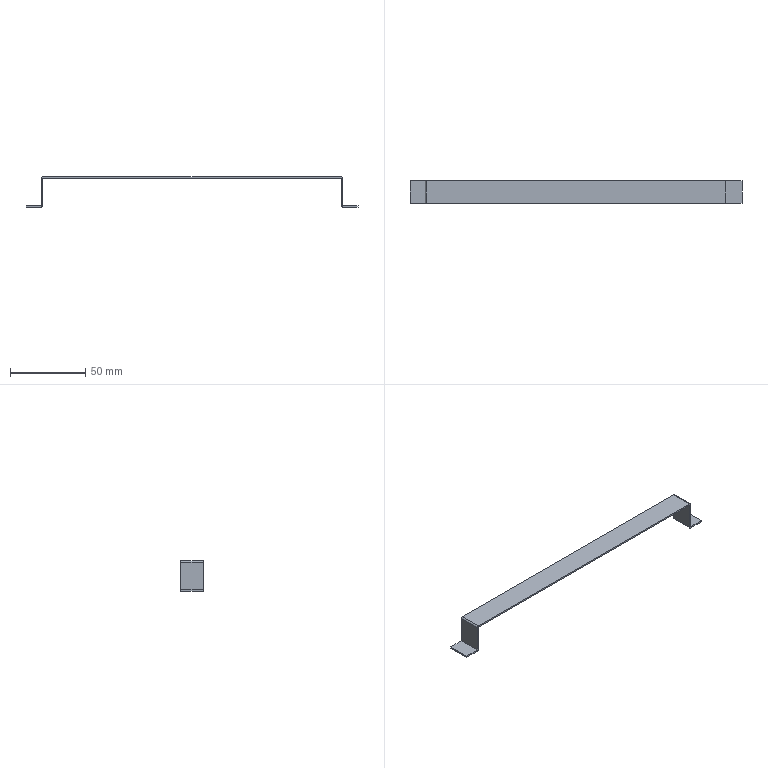Part | STEP file | RJWD-DY-0101_0003 | 1 solid | 18 faces | box 220 x 15 x 20 mm | volume 3858 mm3 | plane 14 | cylinder 4 | commonest cylinder face diameters 2.004 x4
STEP:
#1=CARTESIAN_POINT('',(0.,0.,0.));
#2=DIRECTION('',(0.,0.,1.));
#3=DIRECTION('',(1.,0.,0.));
#4=AXIS2_PLACEMENT_3D('',#1,#2,#3);
#5=CARTESIAN_POINT('',(-779.572,5371.573,97.643));
#6=VERTEX_POINT('',#5);
#7=CARTESIAN_POINT('',(-779.573,5371.573,79.646));
#8=VERTEX_POINT('',#7);
#9=CARTESIAN_POINT('',(-779.572,5371.573,97.643));
#10=DIRECTION('',(-0.00003704,0.,-1.));
#11=VECTOR('',#10,1.);
#12=LINE('',#9,#11);
#13=CARTESIAN_POINT('',(-560.573,5371.573,97.644));
#14=DIRECTION('',(0.,-1.,0.));
#15=DIRECTION('',(0.,0.,-1.));
#16=AXIS2_PLACEMENT_3D('',#13,#14,#15);
#17=PLANE('',#16);
#18=CARTESIAN_POINT('',(0.0006667,-218.999));
#19=DIRECTION('',(1.,-0.00003704));
#20=VECTOR('',#19,1.);
#21=LINE('',#18,#20);
#22=(GEOMETRIC_REPRESENTATION_CONTEXT(2)PARAMETRIC_REPRESENTATION_CONTEXT()REPRESENTATION_CONTEXT('',''));
#23=DEFINITIONAL_REPRESENTATION('',(#21),#22);
#24=PCURVE('',#17,#23);
#25=CARTESIAN_POINT('',(-779.573,-10.,0.));
#26=DIRECTION('',(-1.,0.,0.));
#27=DIRECTION('',(0.,0.,-1.));
#28=AXIS2_PLACEMENT_3D('',#25,#26,#27);
#29=PLANE('',#28);
#30=CARTESIAN_POINT('',(-97.643,-5381.573));
#31=DIRECTION('',(1.,0.));
#32=VECTOR('',#31,1.);
#33=LINE('',#30,#32);
#34=(GEOMETRIC_REPRESENTATION_CONTEXT(2)PARAMETRIC_REPRESENTATION_CONTEXT()REPRESENTATION_CONTEXT('',''));
#35=DEFINITIONAL_REPRESENTATION('',(#33),#34);
#36=PCURVE('',#29,#35);
#37=SURFACE_CURVE('',#12,(#24,#36),.PCURVE_S1.);
#38=EDGE_CURVE('',#6,#8,#37,.T.);
#39=ORIENTED_EDGE('',*,*,#38,.T.);
#40=CARTESIAN_POINT('',(-780.575,5371.573,78.644));
#41=VERTEX_POINT('',#40);
#42=CARTESIAN_POINT('',(-780.575,5371.573,79.646));
#43=DIRECTION('',(0.,-1.,0.));
#44=DIRECTION('',(0.,0.,-1.));
#45=AXIS2_PLACEMENT_3D('',#42,#43,#44);
#46=CIRCLE('',#45,1.002);
#47=CARTESIAN_POINT('',(17.998,-220.002));
#48=DIRECTION('',(1.,0.));
#49=AXIS2_PLACEMENT_2D('',#47,#48);
#50=CIRCLE('',#49,1.002);
#51=(GEOMETRIC_REPRESENTATION_CONTEXT(2)PARAMETRIC_REPRESENTATION_CONTEXT()REPRESENTATION_CONTEXT('',''));
#52=DEFINITIONAL_REPRESENTATION('',(#50),#51);
#53=PCURVE('',#17,#52);
#54=CARTESIAN_POINT('',(-780.575,5411.573,79.646));
#55=DIRECTION('',(0.,-1.,0.));
#56=DIRECTION('',(-1.,0.,0.));
#57=AXIS2_PLACEMENT_3D('',#54,#55,#56);
#58=CYLINDRICAL_SURFACE('',#57,1.002);
#59=CARTESIAN_POINT('',(1.571,40.));
#60=DIRECTION('',(1.,0.));
#61=VECTOR('',#60,1.);
#62=LINE('',#59,#61);
#63=(GEOMETRIC_REPRESENTATION_CONTEXT(2)PARAMETRIC_REPRESENTATION_CONTEXT()REPRESENTATION_CONTEXT('',''));
#64=DEFINITIONAL_REPRESENTATION('',(#62),#63);
#65=PCURVE('',#58,#64);
#66=SURFACE_CURVE('',#46,(#53,#65),.PCURVE_S1.);
#67=EDGE_CURVE('',#41,#8,#66,.T.);
#68=ORIENTED_EDGE('',*,*,#67,.F.);
#69=CARTESIAN_POINT('',(-790.573,5371.573,78.644));
#70=VERTEX_POINT('',#69);
#71=CARTESIAN_POINT('',(-780.575,5371.573,78.644));
#72=DIRECTION('',(-1.,0.,0.));
#73=VECTOR('',#72,1.);
#74=LINE('',#71,#73);
#75=CARTESIAN_POINT('',(19.,-220.002));
#76=DIRECTION('',(0.,-1.));
#77=VECTOR('',#76,1.);
#78=LINE('',#75,#77);
#79=(GEOMETRIC_REPRESENTATION_CONTEXT(2)PARAMETRIC_REPRESENTATION_CONTEXT()REPRESENTATION_CONTEXT('',''));
#80=DEFINITIONAL_REPRESENTATION('',(#78),#79);
#81=PCURVE('',#17,#80);
#82=CARTESIAN_POINT('',(-1601.145,-10.,78.644));
#83=DIRECTION('',(0.,0.,1.));
#84=DIRECTION('',(-1.,0.,0.));
#85=AXIS2_PLACEMENT_3D('',#82,#83,#84);
#86=PLANE('',#85);
#87=CARTESIAN_POINT('',(-820.571,-5381.573));
#88=DIRECTION('',(1.,0.));
#89=VECTOR('',#88,1.);
#90=LINE('',#87,#89);
#91=(GEOMETRIC_REPRESENTATION_CONTEXT(2)PARAMETRIC_REPRESENTATION_CONTEXT()REPRESENTATION_CONTEXT('',''));
#92=DEFINITIONAL_REPRESENTATION('',(#90),#91);
#93=PCURVE('',#86,#92);
#94=SURFACE_CURVE('',#74,(#81,#93),.PCURVE_S1.);
#95=EDGE_CURVE('',#41,#70,#94,.T.);
#96=ORIENTED_EDGE('',*,*,#95,.T.);
#97=CARTESIAN_POINT('',(-790.573,5371.573,79.644));
#98=VERTEX_POINT('',#97);
#99=CARTESIAN_POINT('',(-790.573,5371.573,78.644));
#100=DIRECTION('',(0.,0.,1.));
#101=VECTOR('',#100,1.);
#102=LINE('',#99,#101);
#103=CARTESIAN_POINT('',(19.,-230.));
#104=DIRECTION('',(-1.,0.));
#105=VECTOR('',#104,1.);
#106=LINE('',#103,#105);
#107=(GEOMETRIC_REPRESENTATION_CONTEXT(2)PARAMETRIC_REPRESENTATION_CONTEXT()REPRESENTATION_CONTEXT('',''));
#108=DEFINITIONAL_REPRESENTATION('',(#106),#107);
#109=PCURVE('',#17,#108);
#110=CARTESIAN_POINT('',(-790.573,5371.573,78.644));
#111=DIRECTION('',(-1.,0.,0.));
#112=DIRECTION('',(0.,0.,-1.));
#113=AXIS2_PLACEMENT_3D('',#110,#111,#112);
#114=PLANE('',#113);
#115=CARTESIAN_POINT('',(0.,0.));
#116=DIRECTION('',(-1.,0.));
#117=VECTOR('',#116,1.);
#118=LINE('',#115,#117);
#119=(GEOMETRIC_REPRESENTATION_CONTEXT(2)PARAMETRIC_REPRESENTATION_CONTEXT()REPRESENTATION_CONTEXT('',''));
#120=DEFINITIONAL_REPRESENTATION('',(#118),#119);
#121=PCURVE('',#114,#120);
#122=SURFACE_CURVE('',#102,(#109,#121),.PCURVE_S1.);
#123=EDGE_CURVE('',#70,#98,#122,.T.);
#124=ORIENTED_EDGE('',*,*,#123,.T.);
#125=CARTESIAN_POINT('',(-780.573,5371.573,79.644));
#126=VERTEX_POINT('',#125);
#127=CARTESIAN_POINT('',(-780.573,5371.573,79.644));
#128=DIRECTION('',(-1.,0.,-0.00006667));
#129=VECTOR('',#128,1.);
#130=LINE('',#127,#129);
#131=CARTESIAN_POINT('',(17.999,-220.001));
#132=DIRECTION('',(0.00006667,-1.));
#133=VECTOR('',#132,1.);
#134=LINE('',#131,#133);
#135=(GEOMETRIC_REPRESENTATION_CONTEXT(2)PARAMETRIC_REPRESENTATION_CONTEXT()REPRESENTATION_CONTEXT('',''));
#136=DEFINITIONAL_REPRESENTATION('',(#134),#135);
#137=PCURVE('',#17,#136);
#138=CARTESIAN_POINT('',(-1601.145,-10.,79.644));
#139=DIRECTION('',(0.,0.,1.));
#140=DIRECTION('',(-1.,0.,0.));
#141=AXIS2_PLACEMENT_3D('',#138,#139,#140);
#142=PLANE('',#141);
#143=CARTESIAN_POINT('',(-820.572,-5381.573));
#144=DIRECTION('',(1.,0.));
#145=VECTOR('',#144,1.);
#146=LINE('',#143,#145);
#147=(GEOMETRIC_REPRESENTATION_CONTEXT(2)PARAMETRIC_REPRESENTATION_CONTEXT()REPRESENTATION_CONTEXT('',''));
#148=DEFINITIONAL_REPRESENTATION('',(#146),#147);
#149=PCURVE('',#142,#148);
#150=SURFACE_CURVE('',#130,(#137,#149),.PCURVE_S1.);
#151=EDGE_CURVE('',#126,#98,#150,.T.);
#152=ORIENTED_EDGE('',*,*,#151,.F.);
#153=CARTESIAN_POINT('',(-780.573,5371.573,97.642));
#154=VERTEX_POINT('',#153);
#155=CARTESIAN_POINT('',(-780.573,5371.573,97.642));
#156=DIRECTION('',(-0.00003704,0.,-1.));
#157=VECTOR('',#156,1.);
#158=LINE('',#155,#157);
#159=CARTESIAN_POINT('',(0.002,-220.));
#160=DIRECTION('',(1.,-0.00003704));
#161=VECTOR('',#160,1.);
#162=LINE('',#159,#161);
#163=(GEOMETRIC_REPRESENTATION_CONTEXT(2)PARAMETRIC_REPRESENTATION_CONTEXT()REPRESENTATION_CONTEXT('',''));
#164=DEFINITIONAL_REPRESENTATION('',(#162),#163);
#165=PCURVE('',#17,#164);
#166=CARTESIAN_POINT('',(-780.573,-10.,0.));
#167=DIRECTION('',(-1.,0.,0.));
#168=DIRECTION('',(0.,0.,-1.));
#169=AXIS2_PLACEMENT_3D('',#166,#167,#168);
#170=PLANE('',#169);
#171=CARTESIAN_POINT('',(-97.642,-5381.573));
#172=DIRECTION('',(1.,0.));
#173=VECTOR('',#172,1.);
#174=LINE('',#171,#173);
#175=(GEOMETRIC_REPRESENTATION_CONTEXT(2)PARAMETRIC_REPRESENTATION_CONTEXT()REPRESENTATION_CONTEXT('',''));
#176=DEFINITIONAL_REPRESENTATION('',(#174),#175);
#177=PCURVE('',#170,#176);
#178=SURFACE_CURVE('',#158,(#165,#177),.PCURVE_S1.);
#179=EDGE_CURVE('',#154,#126,#178,.T.);
#180=ORIENTED_EDGE('',*,*,#179,.F.);
#181=CARTESIAN_POINT('',(-779.571,5371.573,98.644));
#182=VERTEX_POINT('',#181);
#183=CARTESIAN_POINT('',(-779.571,5371.573,97.642));
#184=DIRECTION('',(0.,-1.,0.));
#185=DIRECTION('',(0.,0.,1.));
#186=AXIS2_PLACEMENT_3D('',#183,#184,#185);
#187=CIRCLE('',#186,1.002);
#188=CARTESIAN_POINT('',(0.002,-218.998));
#189=DIRECTION('',(-1.,0.));
#190=AXIS2_PLACEMENT_2D('',#188,#189);
#191=CIRCLE('',#190,1.002);
#192=(GEOMETRIC_REPRESENTATION_CONTEXT(2)PARAMETRIC_REPRESENTATION_CONTEXT()REPRESENTATION_CONTEXT('',''));
#193=DEFINITIONAL_REPRESENTATION('',(#191),#192);
#194=PCURVE('',#17,#193);
#195=CARTESIAN_POINT('',(-779.571,5371.573,97.642));
#196=DIRECTION('',(0.,1.,0.));
#197=DIRECTION('',(0.,0.,-1.));
#198=AXIS2_PLACEMENT_3D('',#195,#196,#197);
#199=CYLINDRICAL_SURFACE('',#198,1.002);
#200=CARTESIAN_POINT('',(3.142,0.));
#201=DIRECTION('',(-1.,0.));
#202=VECTOR('',#201,1.);
#203=LINE('',#200,#202);
#204=(GEOMETRIC_REPRESENTATION_CONTEXT(2)PARAMETRIC_REPRESENTATION_CONTEXT()REPRESENTATION_CONTEXT('',''));
#205=DEFINITIONAL_REPRESENTATION('',(#203),#204);
#206=PCURVE('',#199,#205);
#207=SURFACE_CURVE('',#187,(#194,#206),.PCURVE_S1.);
#208=EDGE_CURVE('',#182,#154,#207,.T.);
#209=ORIENTED_EDGE('',*,*,#208,.F.);
#210=CARTESIAN_POINT('',(-581.575,5371.573,98.644));
#211=VERTEX_POINT('',#210);
#212=CARTESIAN_POINT('',(-581.575,5371.573,98.644));
#213=DIRECTION('',(-1.,0.,0.));
#214=VECTOR('',#213,1.);
#215=LINE('',#212,#214);
#216=CARTESIAN_POINT('',(-1.,-21.002));
#217=DIRECTION('',(0.,-1.));
#218=VECTOR('',#217,1.);
#219=LINE('',#216,#218);
#220=(GEOMETRIC_REPRESENTATION_CONTEXT(2)PARAMETRIC_REPRESENTATION_CONTEXT()REPRESENTATION_CONTEXT('',''));
#221=DEFINITIONAL_REPRESENTATION('',(#219),#220);
#222=PCURVE('',#17,#221);
#223=CARTESIAN_POINT('',(-1601.145,-10.,98.644));
#224=DIRECTION('',(0.,0.,1.));
#225=DIRECTION('',(-1.,0.,0.));
#226=AXIS2_PLACEMENT_3D('',#223,#224,#225);
#227=PLANE('',#226);
#228=CARTESIAN_POINT('',(-1019.571,-5381.573));
#229=DIRECTION('',(1.,0.));
#230=VECTOR('',#229,1.);
#231=LINE('',#228,#230);
#232=(GEOMETRIC_REPRESENTATION_CONTEXT(2)PARAMETRIC_REPRESENTATION_CONTEXT()REPRESENTATION_CONTEXT('',''));
#233=DEFINITIONAL_REPRESENTATION('',(#231),#232);
#234=PCURVE('',#227,#233);
#235=SURFACE_CURVE('',#215,(#222,#234),.PCURVE_S1.);
#236=EDGE_CURVE('',#211,#182,#235,.T.);
#237=ORIENTED_EDGE('',*,*,#236,.F.);
#238=CARTESIAN_POINT('',(-580.573,5371.573,97.642));
#239=VERTEX_POINT('',#238);
#240=CARTESIAN_POINT('',(-581.575,5371.573,97.642));
#241=DIRECTION('',(0.,-1.,0.));
#242=DIRECTION('',(1.,0.,0.));
#243=AXIS2_PLACEMENT_3D('',#240,#241,#242);
#244=CIRCLE('',#243,1.002);
#245=CARTESIAN_POINT('',(0.002,-21.002));
#246=DIRECTION('',(0.,1.));
#247=AXIS2_PLACEMENT_2D('',#245,#246);
#248=CIRCLE('',#247,1.002);
#249=(GEOMETRIC_REPRESENTATION_CONTEXT(2)PARAMETRIC_REPRESENTATION_CONTEXT()REPRESENTATION_CONTEXT('',''));
#250=DEFINITIONAL_REPRESENTATION('',(#248),#249);
#251=PCURVE('',#17,#250);
#252=CARTESIAN_POINT('',(-581.575,5411.573,97.642));
#253=DIRECTION('',(0.,-1.,0.));
#254=DIRECTION('',(0.,0.,-1.));
#255=AXIS2_PLACEMENT_3D('',#252,#253,#254);
#256=CYLINDRICAL_SURFACE('',#255,1.002);
#257=CARTESIAN_POINT('',(1.571,40.));
#258=DIRECTION('',(1.,0.));
#259=VECTOR('',#258,1.);
#260=LINE('',#257,#259);
#261=(GEOMETRIC_REPRESENTATION_CONTEXT(2)PARAMETRIC_REPRESENTATION_CONTEXT()REPRESENTATION_CONTEXT('',''));
#262=DEFINITIONAL_REPRESENTATION('',(#260),#261);
#263=PCURVE('',#256,#262);
#264=SURFACE_CURVE('',#244,(#251,#263),.PCURVE_S1.);
#265=EDGE_CURVE('',#239,#211,#264,.T.);
#266=ORIENTED_EDGE('',*,*,#265,.F.);
#267=CARTESIAN_POINT('',(-580.572,5371.573,79.644));
#268=VERTEX_POINT('',#267);
#269=CARTESIAN_POINT('',(-580.573,5371.573,97.642));
#270=DIRECTION('',(0.00003704,0.,-1.));
#271=VECTOR('',#270,1.);
#272=LINE('',#269,#271);
#273=CARTESIAN_POINT('',(0.002,-20.));
#274=DIRECTION('',(1.,0.00003704));
#275=VECTOR('',#274,1.);
#276=LINE('',#273,#275);
#277=(GEOMETRIC_REPRESENTATION_CONTEXT(2)PARAMETRIC_REPRESENTATION_CONTEXT()REPRESENTATION_CONTEXT('',''));
#278=DEFINITIONAL_REPRESENTATION('',(#276),#277);
#279=PCURVE('',#17,#278);
#280=CARTESIAN_POINT('',(-580.573,-10.,0.));
#281=DIRECTION('',(-1.,0.,0.));
#282=DIRECTION('',(0.,0.,-1.));
#283=AXIS2_PLACEMENT_3D('',#280,#281,#282);
#284=PLANE('',#283);
#285=CARTESIAN_POINT('',(-97.642,-5381.573));
#286=DIRECTION('',(1.,0.));
#287=VECTOR('',#286,1.);
#288=LINE('',#285,#287);
#289=(GEOMETRIC_REPRESENTATION_CONTEXT(2)PARAMETRIC_REPRESENTATION_CONTEXT()REPRESENTATION_CONTEXT('',''));
#290=DEFINITIONAL_REPRESENTATION('',(#288),#289);
#291=PCURVE('',#284,#290);
#292=SURFACE_CURVE('',#272,(#279,#291),.PCURVE_S1.);
#293=EDGE_CURVE('',#239,#268,#292,.T.);
#294=ORIENTED_EDGE('',*,*,#293,.T.);
#295=CARTESIAN_POINT('',(-570.573,5371.573,79.644));
#296=VERTEX_POINT('',#295);
#297=CARTESIAN_POINT('',(-580.572,5371.573,79.644));
#298=DIRECTION('',(1.,0.,-0.00006667));
#299=VECTOR('',#298,1.);
#300=LINE('',#297,#299);
#301=CARTESIAN_POINT('',(17.999,-19.999));
#302=DIRECTION('',(0.00006667,1.));
#303=VECTOR('',#302,1.);
#304=LINE('',#301,#303);
#305=(GEOMETRIC_REPRESENTATION_CONTEXT(2)PARAMETRIC_REPRESENTATION_CONTEXT()REPRESENTATION_CONTEXT('',''));
#306=DEFINITIONAL_REPRESENTATION('',(#304),#305);
#307=PCURVE('',#17,#306);
#308=CARTESIAN_POINT('',(-1621.145,-10.,79.644));
#309=DIRECTION('',(0.,0.,-1.));
#310=DIRECTION('',(1.,0.,0.));
#311=AXIS2_PLACEMENT_3D('',#308,#309,#310);
#312=PLANE('',#311);
#313=CARTESIAN_POINT('',(1040.573,-5381.573));
#314=DIRECTION('',(1.,0.));
#315=VECTOR('',#314,1.);
#316=LINE('',#313,#315);
#317=(GEOMETRIC_REPRESENTATION_CONTEXT(2)PARAMETRIC_REPRESENTATION_CONTEXT()REPRESENTATION_CONTEXT('',''));
#318=DEFINITIONAL_REPRESENTATION('',(#316),#317);
#319=PCURVE('',#312,#318);
#320=SURFACE_CURVE('',#300,(#307,#319),.PCURVE_S1.);
#321=EDGE_CURVE('',#268,#296,#320,.T.);
#322=ORIENTED_EDGE('',*,*,#321,.T.);
#323=CARTESIAN_POINT('',(-570.573,5371.573,78.644));
#324=VERTEX_POINT('',#323);
#325=CARTESIAN_POINT('',(-570.573,5371.573,78.644));
#326=DIRECTION('',(0.,0.,1.));
#327=VECTOR('',#326,1.);
#328=LINE('',#325,#327);
#329=CARTESIAN_POINT('',(19.,-10.));
#330=DIRECTION('',(-1.,0.));
#331=VECTOR('',#330,1.);
#332=LINE('',#329,#331);
#333=(GEOMETRIC_REPRESENTATION_CONTEXT(2)PARAMETRIC_REPRESENTATION_CONTEXT()REPRESENTATION_CONTEXT('',''));
#334=DEFINITIONAL_REPRESENTATION('',(#332),#333);
#335=PCURVE('',#17,#334);
#336=CARTESIAN_POINT('',(-570.573,5371.573,78.644));
#337=DIRECTION('',(-1.,0.,0.));
#338=DIRECTION('',(0.,0.,-1.));
#339=AXIS2_PLACEMENT_3D('',#336,#337,#338);
#340=PLANE('',#339);
#341=CARTESIAN_POINT('',(0.,0.));
#342=DIRECTION('',(-1.,0.));
#343=VECTOR('',#342,1.);
#344=LINE('',#341,#343);
#345=(GEOMETRIC_REPRESENTATION_CONTEXT(2)PARAMETRIC_REPRESENTATION_CONTEXT()REPRESENTATION_CONTEXT('',''));
#346=DEFINITIONAL_REPRESENTATION('',(#344),#345);
#347=PCURVE('',#340,#346);
#348=SURFACE_CURVE('',#328,(#335,#347),.PCURVE_S1.);
#349=EDGE_CURVE('',#324,#296,#348,.T.);
#350=ORIENTED_EDGE('',*,*,#349,.F.);
#351=CARTESIAN_POINT('',(-580.571,5371.573,78.644));
#352=VERTEX_POINT('',#351);
#353=CARTESIAN_POINT('',(-580.571,5371.573,78.644));
#354=DIRECTION('',(1.,0.,0.));
#355=VECTOR('',#354,1.);
#356=LINE('',#353,#355);
#357=CARTESIAN_POINT('',(19.,-19.998));
#358=DIRECTION('',(0.,1.));
#359=VECTOR('',#358,1.);
#360=LINE('',#357,#359);
#361=(GEOMETRIC_REPRESENTATION_CONTEXT(2)PARAMETRIC_REPRESENTATION_CONTEXT()REPRESENTATION_CONTEXT('',''));
#362=DEFINITIONAL_REPRESENTATION('',(#360),#361);
#363=PCURVE('',#17,#362);
#364=CARTESIAN_POINT('',(-1621.145,-10.,78.644));
#365=DIRECTION('',(0.,0.,-1.));
#366=DIRECTION('',(1.,0.,0.));
#367=AXIS2_PLACEMENT_3D('',#364,#365,#366);
#368=PLANE('',#367);
#369=CARTESIAN_POINT('',(1040.575,-5381.573));
#370=DIRECTION('',(1.,0.));
#371=VECTOR('',#370,1.);
#372=LINE('',#369,#371);
#373=(GEOMETRIC_REPRESENTATION_CONTEXT(2)PARAMETRIC_REPRESENTATION_CONTEXT()REPRESENTATION_CONTEXT('',''));
#374=DEFINITIONAL_REPRESENTATION('',(#372),#373);
#375=PCURVE('',#368,#374);
#376=SURFACE_CURVE('',#356,(#363,#375),.PCURVE_S1.);
#377=EDGE_CURVE('',#352,#324,#376,.T.);
#378=ORIENTED_EDGE('',*,*,#377,.F.);
#379=CARTESIAN_POINT('',(-581.573,5371.573,79.646));
#380=VERTEX_POINT('',#379);
#381=CARTESIAN_POINT('',(-580.571,5371.573,79.646));
#382=DIRECTION('',(0.,-1.,0.));
#383=DIRECTION('',(-1.,0.,0.));
#384=AXIS2_PLACEMENT_3D('',#381,#382,#383);
#385=CIRCLE('',#384,1.002);
#386=CARTESIAN_POINT('',(17.998,-19.998));
#387=DIRECTION('',(0.,-1.));
#388=AXIS2_PLACEMENT_2D('',#386,#387);
#389=CIRCLE('',#388,1.002);
#390=(GEOMETRIC_REPRESENTATION_CONTEXT(2)PARAMETRIC_REPRESENTATION_CONTEXT()REPRESENTATION_CONTEXT('',''));
#391=DEFINITIONAL_REPRESENTATION('',(#389),#390);
#392=PCURVE('',#17,#391);
#393=CARTESIAN_POINT('',(-580.571,5371.573,79.646));
#394=DIRECTION('',(0.,1.,0.));
#395=DIRECTION('',(1.,0.,0.));
#396=AXIS2_PLACEMENT_3D('',#393,#394,#395);
#397=CYLINDRICAL_SURFACE('',#396,1.002);
#398=CARTESIAN_POINT('',(3.142,0.));
#399=DIRECTION('',(-1.,0.));
#400=VECTOR('',#399,1.);
#401=LINE('',#398,#400);
#402=(GEOMETRIC_REPRESENTATION_CONTEXT(2)PARAMETRIC_REPRESENTATION_CONTEXT()REPRESENTATION_CONTEXT('',''));
#403=DEFINITIONAL_REPRESENTATION('',(#401),#402);
#404=PCURVE('',#397,#403);
#405=SURFACE_CURVE('',#385,(#392,#404),.PCURVE_S1.);
#406=EDGE_CURVE('',#380,#352,#405,.T.);
#407=ORIENTED_EDGE('',*,*,#406,.F.);
#408=CARTESIAN_POINT('',(-581.573,5371.573,97.643));
#409=VERTEX_POINT('',#408);
#410=CARTESIAN_POINT('',(-581.573,5371.573,97.643));
#411=DIRECTION('',(0.00003704,0.,-1.));
#412=VECTOR('',#411,1.);
#413=LINE('',#410,#412);
#414=CARTESIAN_POINT('',(0.0006667,-21.001));
#415=DIRECTION('',(1.,0.00003704));
#416=VECTOR('',#415,1.);
#417=LINE('',#414,#416);
#418=(GEOMETRIC_REPRESENTATION_CONTEXT(2)PARAMETRIC_REPRESENTATION_CONTEXT()REPRESENTATION_CONTEXT('',''));
#419=DEFINITIONAL_REPRESENTATION('',(#417),#418);
#420=PCURVE('',#17,#419);
#421=CARTESIAN_POINT('',(-581.573,-10.,0.));
#422=DIRECTION('',(-1.,0.,0.));
#423=DIRECTION('',(0.,0.,-1.));
#424=AXIS2_PLACEMENT_3D('',#421,#422,#423);
#425=PLANE('',#424);
#426=CARTESIAN_POINT('',(-97.643,-5381.573));
#427=DIRECTION('',(1.,0.));
#428=VECTOR('',#427,1.);
#429=LINE('',#426,#428);
#430=(GEOMETRIC_REPRESENTATION_CONTEXT(2)PARAMETRIC_REPRESENTATION_CONTEXT()REPRESENTATION_CONTEXT('',''));
#431=DEFINITIONAL_REPRESENTATION('',(#429),#430);
#432=PCURVE('',#425,#431);
#433=SURFACE_CURVE('',#413,(#420,#432),.PCURVE_S1.);
#434=EDGE_CURVE('',#409,#380,#433,.T.);
#435=ORIENTED_EDGE('',*,*,#434,.F.);
#436=CARTESIAN_POINT('',(-581.573,5371.573,97.643));
#437=DIRECTION('',(-1.,0.,0.));
#438=VECTOR('',#437,1.);
#439=LINE('',#436,#438);
#440=CARTESIAN_POINT('',(0.0006667,-21.001));
#441=DIRECTION('',(0.,-1.));
#442=VECTOR('',#441,1.);
#443=LINE('',#440,#442);
#444=(GEOMETRIC_REPRESENTATION_CONTEXT(2)PARAMETRIC_REPRESENTATION_CONTEXT()REPRESENTATION_CONTEXT('',''));
#445=DEFINITIONAL_REPRESENTATION('',(#443),#444);
#446=PCURVE('',#17,#445);
#447=CARTESIAN_POINT('',(-1601.145,-10.,97.644));
#448=DIRECTION('',(0.,0.,1.));
#449=DIRECTION('',(-1.,0.,0.));
#450=AXIS2_PLACEMENT_3D('',#447,#448,#449);
#451=PLANE('',#450);
#452=CARTESIAN_POINT('',(-1019.572,-5381.573));
#453=DIRECTION('',(1.,0.));
#454=VECTOR('',#453,1.);
#455=LINE('',#452,#454);
#456=(GEOMETRIC_REPRESENTATION_CONTEXT(2)PARAMETRIC_REPRESENTATION_CONTEXT()REPRESENTATION_CONTEXT('',''));
#457=DEFINITIONAL_REPRESENTATION('',(#455),#456);
#458=PCURVE('',#451,#457);
#459=SURFACE_CURVE('',#439,(#446,#458),.PCURVE_S1.);
#460=EDGE_CURVE('',#409,#6,#459,.T.);
#461=ORIENTED_EDGE('',*,*,#460,.T.);
#462=EDGE_LOOP('',(#39,#68,#96,#124,#152,#180,#209,#237,#266,#294,#322,#350,#378,#407,#435,#461));
#463=FACE_BOUND('',#462,.F.);
#464=ADVANCED_FACE('',(#463),#17,.T.);
#465=CARTESIAN_POINT('',(-779.573,5386.573,79.646));
#466=VERTEX_POINT('',#465);
#467=CARTESIAN_POINT('',(-779.573,5386.573,97.644));
#468=VERTEX_POINT('',#467);
#469=CARTESIAN_POINT('',(-779.573,5386.573,79.646));
#470=DIRECTION('',(0.,0.,1.));
#471=VECTOR('',#470,1.);
#472=LINE('',#469,#471);
#473=CARTESIAN_POINT('',(-79.646,-5396.573));
#474=DIRECTION('',(-1.,0.));
#475=VECTOR('',#474,1.);
#476=LINE('',#473,#475);
#477=(GEOMETRIC_REPRESENTATION_CONTEXT(2)PARAMETRIC_REPRESENTATION_CONTEXT()REPRESENTATION_CONTEXT('',''));
#478=DEFINITIONAL_REPRESENTATION('',(#476),#477);
#479=PCURVE('',#29,#478);
#480=CARTESIAN_POINT('',(-780.573,5386.573,97.644));
#481=DIRECTION('',(0.,1.,0.));
#482=DIRECTION('',(0.,0.,1.));
#483=AXIS2_PLACEMENT_3D('',#480,#481,#482);
#484=PLANE('',#483);
#485=CARTESIAN_POINT('',(-17.998,1.));
#486=DIRECTION('',(1.,0.));
#487=VECTOR('',#486,1.);
#488=LINE('',#485,#487);
#489=(GEOMETRIC_REPRESENTATION_CONTEXT(2)PARAMETRIC_REPRESENTATION_CONTEXT()REPRESENTATION_CONTEXT('',''));
#490=DEFINITIONAL_REPRESENTATION('',(#488),#489);
#491=PCURVE('',#484,#490);
#492=SURFACE_CURVE('',#472,(#479,#491),.PCURVE_S1.);
#493=EDGE_CURVE('',#466,#468,#492,.T.);
#494=ORIENTED_EDGE('',*,*,#493,.F.);
#495=CARTESIAN_POINT('',(-779.573,5386.573,79.646));
#496=DIRECTION('',(0.,-1.,0.));
#497=VECTOR('',#496,1.);
#498=LINE('',#495,#497);
#499=CARTESIAN_POINT('',(-79.646,-5396.573));
#500=DIRECTION('',(0.,1.));
#501=VECTOR('',#500,1.);
#502=LINE('',#499,#501);
#503=(GEOMETRIC_REPRESENTATION_CONTEXT(2)PARAMETRIC_REPRESENTATION_CONTEXT()REPRESENTATION_CONTEXT('',''));
#504=DEFINITIONAL_REPRESENTATION('',(#502),#503);
#505=PCURVE('',#29,#504);
#506=CARTESIAN_POINT('',(3.142,25.));
#507=DIRECTION('',(0.,1.));
#508=VECTOR('',#507,1.);
#509=LINE('',#506,#508);
#510=(GEOMETRIC_REPRESENTATION_CONTEXT(2)PARAMETRIC_REPRESENTATION_CONTEXT()REPRESENTATION_CONTEXT('',''));
#511=DEFINITIONAL_REPRESENTATION('',(#509),#510);
#512=PCURVE('',#58,#511);
#513=SURFACE_CURVE('',#498,(#505,#512),.PCURVE_S1.);
#514=EDGE_CURVE('',#466,#8,#513,.T.);
#515=ORIENTED_EDGE('',*,*,#514,.T.);
#516=ORIENTED_EDGE('',*,*,#38,.F.);
#517=CARTESIAN_POINT('',(-779.572,5371.573,97.643));
#518=DIRECTION('',(-0.00004444,1.,0.00004444));
#519=VECTOR('',#518,1.);
#520=LINE('',#517,#519);
#521=CARTESIAN_POINT('',(-97.643,-5381.573));
#522=DIRECTION('',(-0.00004444,-1.));
#523=VECTOR('',#522,1.);
#524=LINE('',#521,#523);
#525=(GEOMETRIC_REPRESENTATION_CONTEXT(2)PARAMETRIC_REPRESENTATION_CONTEXT()REPRESENTATION_CONTEXT('',''));
#526=DEFINITIONAL_REPRESENTATION('',(#524),#525);
#527=PCURVE('',#29,#526);
#528=CARTESIAN_POINT('',(-821.573,-5381.573));
#529=DIRECTION('',(0.00004444,-1.));
#530=VECTOR('',#529,1.);
#531=LINE('',#528,#530);
#532=(GEOMETRIC_REPRESENTATION_CONTEXT(2)PARAMETRIC_REPRESENTATION_CONTEXT()REPRESENTATION_CONTEXT('',''));
#533=DEFINITIONAL_REPRESENTATION('',(#531),#532);
#534=PCURVE('',#451,#533);
#535=SURFACE_CURVE('',#520,(#527,#534),.PCURVE_S1.);
#536=EDGE_CURVE('',#6,#468,#535,.T.);
#537=ORIENTED_EDGE('',*,*,#536,.T.);
#538=EDGE_LOOP('',(#494,#515,#516,#537));
#539=FACE_BOUND('',#538,.F.);
#540=ADVANCED_FACE('',(#539),#29,.F.);
#541=CARTESIAN_POINT('',(-780.573,5386.573,79.644));
#542=VERTEX_POINT('',#541);
#543=CARTESIAN_POINT('',(-780.573,5386.573,97.642));
#544=VERTEX_POINT('',#543);
#545=CARTESIAN_POINT('',(-780.573,5386.573,79.644));
#546=DIRECTION('',(0.,0.,1.));
#547=VECTOR('',#546,1.);
#548=LINE('',#545,#547);
#549=CARTESIAN_POINT('',(-18.,0.));
#550=DIRECTION('',(1.,0.));
#551=VECTOR('',#550,1.);
#552=LINE('',#549,#551);
#553=(GEOMETRIC_REPRESENTATION_CONTEXT(2)PARAMETRIC_REPRESENTATION_CONTEXT()REPRESENTATION_CONTEXT('',''));
#554=DEFINITIONAL_REPRESENTATION('',(#552),#553);
#555=PCURVE('',#484,#554);
#556=CARTESIAN_POINT('',(-79.644,-5396.573));
#557=DIRECTION('',(-1.,0.));
#558=VECTOR('',#557,1.);
#559=LINE('',#556,#558);
#560=(GEOMETRIC_REPRESENTATION_CONTEXT(2)PARAMETRIC_REPRESENTATION_CONTEXT()REPRESENTATION_CONTEXT('',''));
#561=DEFINITIONAL_REPRESENTATION('',(#559),#560);
#562=PCURVE('',#170,#561);
#563=SURFACE_CURVE('',#548,(#555,#562),.PCURVE_S1.);
#564=EDGE_CURVE('',#542,#544,#563,.T.);
#565=ORIENTED_EDGE('',*,*,#564,.F.);
#566=CARTESIAN_POINT('',(-790.573,5386.573,79.644));
#567=VERTEX_POINT('',#566);
#568=CARTESIAN_POINT('',(-790.573,5386.573,79.644));
#569=DIRECTION('',(1.,0.,0.));
#570=VECTOR('',#569,1.);
#571=LINE('',#568,#570);
#572=CARTESIAN_POINT('',(-18.,-10.));
#573=DIRECTION('',(0.,1.));
#574=VECTOR('',#573,1.);
#575=LINE('',#572,#574);
#576=(GEOMETRIC_REPRESENTATION_CONTEXT(2)PARAMETRIC_REPRESENTATION_CONTEXT()REPRESENTATION_CONTEXT('',''));
#577=DEFINITIONAL_REPRESENTATION('',(#575),#576);
#578=PCURVE('',#484,#577);
#579=CARTESIAN_POINT('',(-810.573,-5396.573));
#580=DIRECTION('',(-1.,0.));
#581=VECTOR('',#580,1.);
#582=LINE('',#579,#581);
#583=(GEOMETRIC_REPRESENTATION_CONTEXT(2)PARAMETRIC_REPRESENTATION_CONTEXT()REPRESENTATION_CONTEXT('',''));
#584=DEFINITIONAL_REPRESENTATION('',(#582),#583);
#585=PCURVE('',#142,#584);
#586=SURFACE_CURVE('',#571,(#578,#585),.PCURVE_S1.);
#587=EDGE_CURVE('',#567,#542,#586,.T.);
#588=ORIENTED_EDGE('',*,*,#587,.F.);
#589=CARTESIAN_POINT('',(-790.573,5386.573,78.644));
#590=VERTEX_POINT('',#589);
#591=CARTESIAN_POINT('',(-790.573,5386.573,78.644));
#592=DIRECTION('',(0.,0.,1.));
#593=VECTOR('',#592,1.);
#594=LINE('',#591,#593);
#595=CARTESIAN_POINT('',(-19.,-10.));
#596=DIRECTION('',(1.,0.));
#597=VECTOR('',#596,1.);
#598=LINE('',#595,#597);
#599=(GEOMETRIC_REPRESENTATION_CONTEXT(2)PARAMETRIC_REPRESENTATION_CONTEXT()REPRESENTATION_CONTEXT('',''));
#600=DEFINITIONAL_REPRESENTATION('',(#598),#599);
#601=PCURVE('',#484,#600);
#602=CARTESIAN_POINT('',(0.,-15.));
#603=DIRECTION('',(-1.,0.));
#604=VECTOR('',#603,1.);
#605=LINE('',#602,#604);
#606=(GEOMETRIC_REPRESENTATION_CONTEXT(2)PARAMETRIC_REPRESENTATION_CONTEXT()REPRESENTATION_CONTEXT('',''));
#607=DEFINITIONAL_REPRESENTATION('',(#605),#606);
#608=PCURVE('',#114,#607);
#609=SURFACE_CURVE('',#594,(#601,#608),.PCURVE_S1.);
#610=EDGE_CURVE('',#590,#567,#609,.T.);
#611=ORIENTED_EDGE('',*,*,#610,.F.);
#612=CARTESIAN_POINT('',(-780.575,5386.573,78.644));
#613=VERTEX_POINT('',#612);
#614=CARTESIAN_POINT('',(-790.573,5386.573,78.644));
#615=DIRECTION('',(1.,0.,0.));
#616=VECTOR('',#615,1.);
#617=LINE('',#614,#616);
#618=CARTESIAN_POINT('',(-19.,-10.));
#619=DIRECTION('',(0.,1.));
#620=VECTOR('',#619,1.);
#621=LINE('',#618,#620);
#622=(GEOMETRIC_REPRESENTATION_CONTEXT(2)PARAMETRIC_REPRESENTATION_CONTEXT()REPRESENTATION_CONTEXT('',''));
#623=DEFINITIONAL_REPRESENTATION('',(#621),#622);
#624=PCURVE('',#484,#623);
#625=CARTESIAN_POINT('',(-810.573,-5396.573));
#626=DIRECTION('',(-1.,0.));
#627=VECTOR('',#626,1.);
#628=LINE('',#625,#627);
#629=(GEOMETRIC_REPRESENTATION_CONTEXT(2)PARAMETRIC_REPRESENTATION_CONTEXT()REPRESENTATION_CONTEXT('',''));
#630=DEFINITIONAL_REPRESENTATION('',(#628),#629);
#631=PCURVE('',#86,#630);
#632=SURFACE_CURVE('',#617,(#624,#631),.PCURVE_S1.);
#633=EDGE_CURVE('',#590,#613,#632,.T.);
#634=ORIENTED_EDGE('',*,*,#633,.T.);
#635=CARTESIAN_POINT('',(-780.575,5386.573,79.646));
#636=DIRECTION('',(0.,1.,0.));
#637=DIRECTION('',(1.,0.,0.));
#638=AXIS2_PLACEMENT_3D('',#635,#636,#637);
#639=CIRCLE('',#638,1.002);
#640=CARTESIAN_POINT('',(-17.998,-0.002));
#641=DIRECTION('',(0.,1.));
#642=AXIS2_PLACEMENT_2D('',#640,#641);
#643=CIRCLE('',#642,1.002);
#644=(GEOMETRIC_REPRESENTATION_CONTEXT(2)PARAMETRIC_REPRESENTATION_CONTEXT()REPRESENTATION_CONTEXT('',''));
#645=DEFINITIONAL_REPRESENTATION('',(#643),#644);
#646=PCURVE('',#484,#645);
#647=CARTESIAN_POINT('',(3.142,25.));
#648=DIRECTION('',(-1.,0.));
#649=VECTOR('',#648,1.);
#650=LINE('',#647,#649);
#651=(GEOMETRIC_REPRESENTATION_CONTEXT(2)PARAMETRIC_REPRESENTATION_CONTEXT()REPRESENTATION_CONTEXT('',''));
#652=DEFINITIONAL_REPRESENTATION('',(#650),#651);
#653=PCURVE('',#58,#652);
#654=SURFACE_CURVE('',#639,(#646,#653),.PCURVE_S1.);
#655=EDGE_CURVE('',#466,#613,#654,.T.);
#656=ORIENTED_EDGE('',*,*,#655,.F.);
#657=ORIENTED_EDGE('',*,*,#493,.T.);
#658=CARTESIAN_POINT('',(-581.573,5386.573,97.644));
#659=VERTEX_POINT('',#658);
#660=CARTESIAN_POINT('',(-779.573,5386.573,97.644));
#661=DIRECTION('',(1.,0.,0.));
#662=VECTOR('',#661,1.);
#663=LINE('',#660,#662);
#664=CARTESIAN_POINT('',(0.,1.));
#665=DIRECTION('',(0.,1.));
#666=VECTOR('',#665,1.);
#667=LINE('',#664,#666);
#668=(GEOMETRIC_REPRESENTATION_CONTEXT(2)PARAMETRIC_REPRESENTATION_CONTEXT()REPRESENTATION_CONTEXT('',''));
#669=DEFINITIONAL_REPRESENTATION('',(#667),#668);
#670=PCURVE('',#484,#669);
#671=CARTESIAN_POINT('',(-821.573,-5396.573));
#672=DIRECTION('',(-1.,0.));
#673=VECTOR('',#672,1.);
#674=LINE('',#671,#673);
#675=(GEOMETRIC_REPRESENTATION_CONTEXT(2)PARAMETRIC_REPRESENTATION_CONTEXT()REPRESENTATION_CONTEXT('',''));
#676=DEFINITIONAL_REPRESENTATION('',(#674),#675);
#677=PCURVE('',#451,#676);
#678=SURFACE_CURVE('',#663,(#670,#677),.PCURVE_S1.);
#679=EDGE_CURVE('',#468,#659,#678,.T.);
#680=ORIENTED_EDGE('',*,*,#679,.T.);
#681=CARTESIAN_POINT('',(-581.573,5386.573,79.646));
#682=VERTEX_POINT('',#681);
#683=CARTESIAN_POINT('',(-581.573,5386.573,79.646));
#684=DIRECTION('',(0.,0.,1.));
#685=VECTOR('',#684,1.);
#686=LINE('',#683,#685);
#687=CARTESIAN_POINT('',(-17.998,199.));
#688=DIRECTION('',(1.,0.));
#689=VECTOR('',#688,1.);
#690=LINE('',#687,#689);
#691=(GEOMETRIC_REPRESENTATION_CONTEXT(2)PARAMETRIC_REPRESENTATION_CONTEXT()REPRESENTATION_CONTEXT('',''));
#692=DEFINITIONAL_REPRESENTATION('',(#690),#691);
#693=PCURVE('',#484,#692);
#694=CARTESIAN_POINT('',(-79.646,-5396.573));
#695=DIRECTION('',(-1.,0.));
#696=VECTOR('',#695,1.);
#697=LINE('',#694,#696);
#698=(GEOMETRIC_REPRESENTATION_CONTEXT(2)PARAMETRIC_REPRESENTATION_CONTEXT()REPRESENTATION_CONTEXT('',''));
#699=DEFINITIONAL_REPRESENTATION('',(#697),#698);
#700=PCURVE('',#425,#699);
#701=SURFACE_CURVE('',#686,(#693,#700),.PCURVE_S1.);
#702=EDGE_CURVE('',#682,#659,#701,.T.);
#703=ORIENTED_EDGE('',*,*,#702,.F.);
#704=CARTESIAN_POINT('',(-580.571,5386.573,78.644));
#705=VERTEX_POINT('',#704);
#706=CARTESIAN_POINT('',(-580.571,5386.573,79.646));
#707=DIRECTION('',(0.,1.,0.));
#708=DIRECTION('',(0.,0.,-1.));
#709=AXIS2_PLACEMENT_3D('',#706,#707,#708);
#710=CIRCLE('',#709,1.002);
#711=CARTESIAN_POINT('',(-17.998,200.002));
#712=DIRECTION('',(-1.,0.));
#713=AXIS2_PLACEMENT_2D('',#711,#712);
#714=CIRCLE('',#713,1.002);
#715=(GEOMETRIC_REPRESENTATION_CONTEXT(2)PARAMETRIC_REPRESENTATION_CONTEXT()REPRESENTATION_CONTEXT('',''));
#716=DEFINITIONAL_REPRESENTATION('',(#714),#715);
#717=PCURVE('',#484,#716);
#718=CARTESIAN_POINT('',(1.571,15.));
#719=DIRECTION('',(1.,0.));
#720=VECTOR('',#719,1.);
#721=LINE('',#718,#720);
#722=(GEOMETRIC_REPRESENTATION_CONTEXT(2)PARAMETRIC_REPRESENTATION_CONTEXT()REPRESENTATION_CONTEXT('',''));
#723=DEFINITIONAL_REPRESENTATION('',(#721),#722);
#724=PCURVE('',#397,#723);
#725=SURFACE_CURVE('',#710,(#717,#724),.PCURVE_S1.);
#726=EDGE_CURVE('',#705,#682,#725,.T.);
#727=ORIENTED_EDGE('',*,*,#726,.F.);
#728=CARTESIAN_POINT('',(-570.573,5386.573,78.644));
#729=VERTEX_POINT('',#728);
#730=CARTESIAN_POINT('',(-570.573,5386.573,78.644));
#731=DIRECTION('',(-1.,0.,0.));
#732=VECTOR('',#731,1.);
#733=LINE('',#730,#732);
#734=CARTESIAN_POINT('',(-19.,210.));
#735=DIRECTION('',(0.,-1.));
#736=VECTOR('',#735,1.);
#737=LINE('',#734,#736);
#738=(GEOMETRIC_REPRESENTATION_CONTEXT(2)PARAMETRIC_REPRESENTATION_CONTEXT()REPRESENTATION_CONTEXT('',''));
#739=DEFINITIONAL_REPRESENTATION('',(#737),#738);
#740=PCURVE('',#484,#739);
#741=CARTESIAN_POINT('',(1050.573,-5396.573));
#742=DIRECTION('',(-1.,0.));
#743=VECTOR('',#742,1.);
#744=LINE('',#741,#743);
#745=(GEOMETRIC_REPRESENTATION_CONTEXT(2)PARAMETRIC_REPRESENTATION_CONTEXT()REPRESENTATION_CONTEXT('',''));
#746=DEFINITIONAL_REPRESENTATION('',(#744),#745);
#747=PCURVE('',#368,#746);
#748=SURFACE_CURVE('',#733,(#740,#747),.PCURVE_S1.);
#749=EDGE_CURVE('',#729,#705,#748,.T.);
#750=ORIENTED_EDGE('',*,*,#749,.F.);
#751=CARTESIAN_POINT('',(-570.573,5386.573,79.644));
#752=VERTEX_POINT('',#751);
#753=CARTESIAN_POINT('',(-570.573,5386.573,78.644));
#754=DIRECTION('',(0.,0.,1.));
#755=VECTOR('',#754,1.);
#756=LINE('',#753,#755);
#757=CARTESIAN_POINT('',(-19.,210.));
#758=DIRECTION('',(1.,0.));
#759=VECTOR('',#758,1.);
#760=LINE('',#757,#759);
#761=(GEOMETRIC_REPRESENTATION_CONTEXT(2)PARAMETRIC_REPRESENTATION_CONTEXT()REPRESENTATION_CONTEXT('',''));
#762=DEFINITIONAL_REPRESENTATION('',(#760),#761);
#763=PCURVE('',#484,#762);
#764=CARTESIAN_POINT('',(0.,-15.));
#765=DIRECTION('',(-1.,0.));
#766=VECTOR('',#765,1.);
#767=LINE('',#764,#766);
#768=(GEOMETRIC_REPRESENTATION_CONTEXT(2)PARAMETRIC_REPRESENTATION_CONTEXT()REPRESENTATION_CONTEXT('',''));
#769=DEFINITIONAL_REPRESENTATION('',(#767),#768);
#770=PCURVE('',#340,#769);
#771=SURFACE_CURVE('',#756,(#763,#770),.PCURVE_S1.);
#772=EDGE_CURVE('',#729,#752,#771,.T.);
#773=ORIENTED_EDGE('',*,*,#772,.T.);
#774=CARTESIAN_POINT('',(-580.573,5386.573,79.644));
#775=VERTEX_POINT('',#774);
#776=CARTESIAN_POINT('',(-570.573,5386.573,79.644));
#777=DIRECTION('',(-1.,0.,0.));
#778=VECTOR('',#777,1.);
#779=LINE('',#776,#778);
#780=CARTESIAN_POINT('',(-18.,210.));
#781=DIRECTION('',(0.,-1.));
#782=VECTOR('',#781,1.);
#783=LINE('',#780,#782);
#784=(GEOMETRIC_REPRESENTATION_CONTEXT(2)PARAMETRIC_REPRESENTATION_CONTEXT()REPRESENTATION_CONTEXT('',''));
#785=DEFINITIONAL_REPRESENTATION('',(#783),#784);
#786=PCURVE('',#484,#785);
#787=CARTESIAN_POINT('',(1050.573,-5396.573));
#788=DIRECTION('',(-1.,0.));
#789=VECTOR('',#788,1.);
#790=LINE('',#787,#789);
#791=(GEOMETRIC_REPRESENTATION_CONTEXT(2)PARAMETRIC_REPRESENTATION_CONTEXT()REPRESENTATION_CONTEXT('',''));
#792=DEFINITIONAL_REPRESENTATION('',(#790),#791);
#793=PCURVE('',#312,#792);
#794=SURFACE_CURVE('',#779,(#786,#793),.PCURVE_S1.);
#795=EDGE_CURVE('',#752,#775,#794,.T.);
#796=ORIENTED_EDGE('',*,*,#795,.T.);
#797=CARTESIAN_POINT('',(-580.573,5386.573,97.642));
#798=VERTEX_POINT('',#797);
#799=CARTESIAN_POINT('',(-580.573,5386.573,79.644));
#800=DIRECTION('',(0.,0.,1.));
#801=VECTOR('',#800,1.);
#802=LINE('',#799,#801);
#803=CARTESIAN_POINT('',(-18.,200.));
#804=DIRECTION('',(1.,0.));
#805=VECTOR('',#804,1.);
#806=LINE('',#803,#805);
#807=(GEOMETRIC_REPRESENTATION_CONTEXT(2)PARAMETRIC_REPRESENTATION_CONTEXT()REPRESENTATION_CONTEXT('',''));
#808=DEFINITIONAL_REPRESENTATION('',(#806),#807);
#809=PCURVE('',#484,#808);
#810=CARTESIAN_POINT('',(-79.644,-5396.573));
#811=DIRECTION('',(-1.,0.));
#812=VECTOR('',#811,1.);
#813=LINE('',#810,#812);
#814=(GEOMETRIC_REPRESENTATION_CONTEXT(2)PARAMETRIC_REPRESENTATION_CONTEXT()REPRESENTATION_CONTEXT('',''));
#815=DEFINITIONAL_REPRESENTATION('',(#813),#814);
#816=PCURVE('',#284,#815);
#817=SURFACE_CURVE('',#802,(#809,#816),.PCURVE_S1.);
#818=EDGE_CURVE('',#775,#798,#817,.T.);
#819=ORIENTED_EDGE('',*,*,#818,.T.);
#820=CARTESIAN_POINT('',(-581.575,5386.573,98.644));
#821=VERTEX_POINT('',#820);
#822=CARTESIAN_POINT('',(-581.575,5386.573,97.642));
#823=DIRECTION('',(0.,1.,0.));
#824=DIRECTION('',(0.,0.,1.));
#825=AXIS2_PLACEMENT_3D('',#822,#823,#824);
#826=CIRCLE('',#825,1.002);
#827=CARTESIAN_POINT('',(-0.002,198.998));
#828=DIRECTION('',(1.,0.));
#829=AXIS2_PLACEMENT_2D('',#827,#828);
#830=CIRCLE('',#829,1.002);
#831=(GEOMETRIC_REPRESENTATION_CONTEXT(2)PARAMETRIC_REPRESENTATION_CONTEXT()REPRESENTATION_CONTEXT('',''));
#832=DEFINITIONAL_REPRESENTATION('',(#830),#831);
#833=PCURVE('',#484,#832);
#834=CARTESIAN_POINT('',(3.142,25.));
#835=DIRECTION('',(-1.,0.));
#836=VECTOR('',#835,1.);
#837=LINE('',#834,#836);
#838=(GEOMETRIC_REPRESENTATION_CONTEXT(2)PARAMETRIC_REPRESENTATION_CONTEXT()REPRESENTATION_CONTEXT('',''));
#839=DEFINITIONAL_REPRESENTATION('',(#837),#838);
#840=PCURVE('',#256,#839);
#841=SURFACE_CURVE('',#826,(#833,#840),.PCURVE_S1.);
#842=EDGE_CURVE('',#821,#798,#841,.T.);
#843=ORIENTED_EDGE('',*,*,#842,.F.);
#844=CARTESIAN_POINT('',(-779.571,5386.573,98.644));
#845=VERTEX_POINT('',#844);
#846=CARTESIAN_POINT('',(-779.571,5386.573,98.644));
#847=DIRECTION('',(1.,0.,0.));
#848=VECTOR('',#847,1.);
#849=LINE('',#846,#848);
#850=CARTESIAN_POINT('',(1.,1.002));
#851=DIRECTION('',(0.,1.));
#852=VECTOR('',#851,1.);
#853=LINE('',#850,#852);
#854=(GEOMETRIC_REPRESENTATION_CONTEXT(2)PARAMETRIC_REPRESENTATION_CONTEXT()REPRESENTATION_CONTEXT('',''));
#855=DEFINITIONAL_REPRESENTATION('',(#853),#854);
#856=PCURVE('',#484,#855);
#857=CARTESIAN_POINT('',(-821.575,-5396.573));
#858=DIRECTION('',(-1.,0.));
#859=VECTOR('',#858,1.);
#860=LINE('',#857,#859);
#861=(GEOMETRIC_REPRESENTATION_CONTEXT(2)PARAMETRIC_REPRESENTATION_CONTEXT()REPRESENTATION_CONTEXT('',''));
#862=DEFINITIONAL_REPRESENTATION('',(#860),#861);
#863=PCURVE('',#227,#862);
#864=SURFACE_CURVE('',#849,(#856,#863),.PCURVE_S1.);
#865=EDGE_CURVE('',#845,#821,#864,.T.);
#866=ORIENTED_EDGE('',*,*,#865,.F.);
#867=CARTESIAN_POINT('',(-779.571,5386.573,97.642));
#868=DIRECTION('',(0.,1.,0.));
#869=DIRECTION('',(-1.,0.,0.));
#870=AXIS2_PLACEMENT_3D('',#867,#868,#869);
#871=CIRCLE('',#870,1.002);
#872=CARTESIAN_POINT('',(-0.002,1.002));
#873=DIRECTION('',(0.,-1.));
#874=AXIS2_PLACEMENT_2D('',#872,#873);
#875=CIRCLE('',#874,1.002);
#876=(GEOMETRIC_REPRESENTATION_CONTEXT(2)PARAMETRIC_REPRESENTATION_CONTEXT()REPRESENTATION_CONTEXT('',''));
#877=DEFINITIONAL_REPRESENTATION('',(#875),#876);
#878=PCURVE('',#484,#877);
#879=CARTESIAN_POINT('',(1.571,15.));
#880=DIRECTION('',(1.,0.));
#881=VECTOR('',#880,1.);
#882=LINE('',#879,#881);
#883=(GEOMETRIC_REPRESENTATION_CONTEXT(2)PARAMETRIC_REPRESENTATION_CONTEXT()REPRESENTATION_CONTEXT('',''));
#884=DEFINITIONAL_REPRESENTATION('',(#882),#883);
#885=PCURVE('',#199,#884);
#886=SURFACE_CURVE('',#871,(#878,#885),.PCURVE_S1.);
#887=EDGE_CURVE('',#544,#845,#886,.T.);
#888=ORIENTED_EDGE('',*,*,#887,.F.);
#889=EDGE_LOOP('',(#565,#588,#611,#634,#656,#657,#680,#703,#727,#750,#773,#796,#819,#843,#866,#888));
#890=FACE_BOUND('',#889,.F.);
#891=ADVANCED_FACE('',(#890),#484,.T.);
#892=ORIENTED_EDGE('',*,*,#179,.F.);
#893=CARTESIAN_POINT('',(-780.573,5386.573,97.642));
#894=DIRECTION('',(0.,-1.,0.));
#895=VECTOR('',#894,1.);
#896=LINE('',#893,#895);
#897=CARTESIAN_POINT('',(-97.642,-5396.573));
#898=DIRECTION('',(0.,1.));
#899=VECTOR('',#898,1.);
#900=LINE('',#897,#899);
#901=(GEOMETRIC_REPRESENTATION_CONTEXT(2)PARAMETRIC_REPRESENTATION_CONTEXT()REPRESENTATION_CONTEXT('',''));
#902=DEFINITIONAL_REPRESENTATION('',(#900),#901);
#903=PCURVE('',#170,#902);
#904=CARTESIAN_POINT('',(1.571,15.));
#905=DIRECTION('',(0.,-1.));
#906=VECTOR('',#905,1.);
#907=LINE('',#904,#906);
#908=(GEOMETRIC_REPRESENTATION_CONTEXT(2)PARAMETRIC_REPRESENTATION_CONTEXT()REPRESENTATION_CONTEXT('',''));
#909=DEFINITIONAL_REPRESENTATION('',(#907),#908);
#910=PCURVE('',#199,#909);
#911=SURFACE_CURVE('',#896,(#903,#910),.PCURVE_S1.);
#912=EDGE_CURVE('',#544,#154,#911,.T.);
#913=ORIENTED_EDGE('',*,*,#912,.F.);
#914=ORIENTED_EDGE('',*,*,#564,.F.);
#915=CARTESIAN_POINT('',(-780.573,5371.573,79.644));
#916=DIRECTION('',(0.00004444,1.,-0.00004444));
#917=VECTOR('',#916,1.);
#918=LINE('',#915,#917);
#919=CARTESIAN_POINT('',(-79.644,-5381.573));
#920=DIRECTION('',(0.00004444,-1.));
#921=VECTOR('',#920,1.);
#922=LINE('',#919,#921);
#923=(GEOMETRIC_REPRESENTATION_CONTEXT(2)PARAMETRIC_REPRESENTATION_CONTEXT()REPRESENTATION_CONTEXT('',''));
#924=DEFINITIONAL_REPRESENTATION('',(#922),#923);
#925=PCURVE('',#170,#924);
#926=CARTESIAN_POINT('',(-820.572,-5381.573));
#927=DIRECTION('',(-0.00004444,-1.));
#928=VECTOR('',#927,1.);
#929=LINE('',#926,#928);
#930=(GEOMETRIC_REPRESENTATION_CONTEXT(2)PARAMETRIC_REPRESENTATION_CONTEXT()REPRESENTATION_CONTEXT('',''));
#931=DEFINITIONAL_REPRESENTATION('',(#929),#930);
#932=PCURVE('',#142,#931);
#933=SURFACE_CURVE('',#918,(#925,#932),.PCURVE_S1.);
#934=EDGE_CURVE('',#126,#542,#933,.T.);
#935=ORIENTED_EDGE('',*,*,#934,.F.);
#936=EDGE_LOOP('',(#892,#913,#914,#935));
#937=FACE_BOUND('',#936,.T.);
#938=ADVANCED_FACE('',(#937),#170,.T.);
#939=ORIENTED_EDGE('',*,*,#587,.T.);
#940=ORIENTED_EDGE('',*,*,#934,.F.);
#941=ORIENTED_EDGE('',*,*,#151,.T.);
#942=CARTESIAN_POINT('',(-790.573,5371.573,79.644));
#943=DIRECTION('',(0.,1.,0.));
#944=VECTOR('',#943,1.);
#945=LINE('',#942,#944);
#946=CARTESIAN_POINT('',(-810.573,-5381.573));
#947=DIRECTION('',(0.,-1.));
#948=VECTOR('',#947,1.);
#949=LINE('',#946,#948);
#950=(GEOMETRIC_REPRESENTATION_CONTEXT(2)PARAMETRIC_REPRESENTATION_CONTEXT()REPRESENTATION_CONTEXT('',''));
#951=DEFINITIONAL_REPRESENTATION('',(#949),#950);
#952=PCURVE('',#142,#951);
#953=CARTESIAN_POINT('',(-1.,0.));
#954=DIRECTION('',(0.,-1.));
#955=VECTOR('',#954,1.);
#956=LINE('',#953,#955);
#957=(GEOMETRIC_REPRESENTATION_CONTEXT(2)PARAMETRIC_REPRESENTATION_CONTEXT()REPRESENTATION_CONTEXT('',''));
#958=DEFINITIONAL_REPRESENTATION('',(#956),#957);
#959=PCURVE('',#114,#958);
#960=SURFACE_CURVE('',#945,(#952,#959),.PCURVE_S1.);
#961=EDGE_CURVE('',#98,#567,#960,.T.);
#962=ORIENTED_EDGE('',*,*,#961,.T.);
#963=EDGE_LOOP('',(#939,#940,#941,#962));
#964=FACE_BOUND('',#963,.F.);
#965=ADVANCED_FACE('',(#964),#142,.T.);
#966=ORIENTED_EDGE('',*,*,#961,.F.);
#967=ORIENTED_EDGE('',*,*,#123,.F.);
#968=CARTESIAN_POINT('',(-790.573,5371.573,78.644));
#969=DIRECTION('',(0.,1.,0.));
#970=VECTOR('',#969,1.);
#971=LINE('',#968,#970);
#972=CARTESIAN_POINT('',(0.,0.));
#973=DIRECTION('',(0.,-1.));
#974=VECTOR('',#973,1.);
#975=LINE('',#972,#974);
#976=(GEOMETRIC_REPRESENTATION_CONTEXT(2)PARAMETRIC_REPRESENTATION_CONTEXT()REPRESENTATION_CONTEXT('',''));
#977=DEFINITIONAL_REPRESENTATION('',(#975),#976);
#978=PCURVE('',#114,#977);
#979=CARTESIAN_POINT('',(-810.573,-5381.573));
#980=DIRECTION('',(0.,-1.));
#981=VECTOR('',#980,1.);
#982=LINE('',#979,#981);
#983=(GEOMETRIC_REPRESENTATION_CONTEXT(2)PARAMETRIC_REPRESENTATION_CONTEXT()REPRESENTATION_CONTEXT('',''));
#984=DEFINITIONAL_REPRESENTATION('',(#982),#983);
#985=PCURVE('',#86,#984);
#986=SURFACE_CURVE('',#971,(#978,#985),.PCURVE_S1.);
#987=EDGE_CURVE('',#70,#590,#986,.T.);
#988=ORIENTED_EDGE('',*,*,#987,.T.);
#989=ORIENTED_EDGE('',*,*,#610,.T.);
#990=EDGE_LOOP('',(#966,#967,#988,#989));
#991=FACE_BOUND('',#990,.F.);
#992=ADVANCED_FACE('',(#991),#114,.T.);
#993=CARTESIAN_POINT('',(-780.575,5371.573,78.644));
#994=DIRECTION('',(0.,1.,0.));
#995=VECTOR('',#994,1.);
#996=LINE('',#993,#995);
#997=CARTESIAN_POINT('',(-820.571,-5381.573));
#998=DIRECTION('',(0.,-1.));
#999=VECTOR('',#998,1.);
#1000=LINE('',#997,#999);
#1001=(GEOMETRIC_REPRESENTATION_CONTEXT(2)PARAMETRIC_REPRESENTATION_CONTEXT()REPRESENTATION_CONTEXT('',''));
#1002=DEFINITIONAL_REPRESENTATION('',(#1000),#1001);
#1003=PCURVE('',#86,#1002);
#1004=CARTESIAN_POINT('',(1.571,40.));
#1005=DIRECTION('',(0.,-1.));
#1006=VECTOR('',#1005,1.);
#1007=LINE('',#1004,#1006);
#1008=(GEOMETRIC_REPRESENTATION_CONTEXT(2)PARAMETRIC_REPRESENTATION_CONTEXT()REPRESENTATION_CONTEXT('',''));
#1009=DEFINITIONAL_REPRESENTATION('',(#1007),#1008);
#1010=PCURVE('',#58,#1009);
#1011=SURFACE_CURVE('',#996,(#1003,#1010),.PCURVE_S1.);
#1012=EDGE_CURVE('',#41,#613,#1011,.T.);
#1013=ORIENTED_EDGE('',*,*,#1012,.T.);
#1014=ORIENTED_EDGE('',*,*,#633,.F.);
#1015=ORIENTED_EDGE('',*,*,#987,.F.);
#1016=ORIENTED_EDGE('',*,*,#95,.F.);
#1017=EDGE_LOOP('',(#1013,#1014,#1015,#1016));
#1018=FACE_BOUND('',#1017,.F.);
#1019=ADVANCED_FACE('',(#1018),#86,.F.);
#1020=ORIENTED_EDGE('',*,*,#67,.F.);
#1021=ORIENTED_EDGE('',*,*,#1012,.T.);
#1022=ORIENTED_EDGE('',*,*,#655,.F.);
#1023=ORIENTED_EDGE('',*,*,#514,.T.);
#1024=EDGE_LOOP('',(#1020,#1021,#1022,#1023));
#1025=FACE_BOUND('',#1024,.T.);
#1026=ADVANCED_FACE('',(#1025),#58,.T.);
#1027=ORIENTED_EDGE('',*,*,#887,.F.);
#1028=ORIENTED_EDGE('',*,*,#912,.T.);
#1029=ORIENTED_EDGE('',*,*,#208,.F.);
#1030=CARTESIAN_POINT('',(-779.571,5371.573,98.644));
#1031=DIRECTION('',(0.,1.,0.));
#1032=VECTOR('',#1031,1.);
#1033=LINE('',#1030,#1032);
#1034=CARTESIAN_POINT('',(3.142,0.));
#1035=DIRECTION('',(0.,1.));
#1036=VECTOR('',#1035,1.);
#1037=LINE('',#1034,#1036);
#1038=(GEOMETRIC_REPRESENTATION_CONTEXT(2)PARAMETRIC_REPRESENTATION_CONTEXT()REPRESENTATION_CONTEXT('',''));
#1039=DEFINITIONAL_REPRESENTATION('',(#1037),#1038);
#1040=PCURVE('',#199,#1039);
#1041=CARTESIAN_POINT('',(-821.575,-5381.573));
#1042=DIRECTION('',(0.,-1.));
#1043=VECTOR('',#1042,1.);
#1044=LINE('',#1041,#1043);
#1045=(GEOMETRIC_REPRESENTATION_CONTEXT(2)PARAMETRIC_REPRESENTATION_CONTEXT()REPRESENTATION_CONTEXT('',''));
#1046=DEFINITIONAL_REPRESENTATION('',(#1044),#1045);
#1047=PCURVE('',#227,#1046);
#1048=SURFACE_CURVE('',#1033,(#1040,#1047),.PCURVE_S1.);
#1049=EDGE_CURVE('',#182,#845,#1048,.T.);
#1050=ORIENTED_EDGE('',*,*,#1049,.T.);
#1051=EDGE_LOOP('',(#1027,#1028,#1029,#1050));
#1052=FACE_BOUND('',#1051,.T.);
#1053=ADVANCED_FACE('',(#1052),#199,.T.);
#1054=ORIENTED_EDGE('',*,*,#865,.T.);
#1055=CARTESIAN_POINT('',(-581.575,5386.573,98.644));
#1056=DIRECTION('',(0.,-1.,0.));
#1057=VECTOR('',#1056,1.);
#1058=LINE('',#1055,#1057);
#1059=CARTESIAN_POINT('',(-1019.571,-5396.573));
#1060=DIRECTION('',(0.,1.));
#1061=VECTOR('',#1060,1.);
#1062=LINE('',#1059,#1061);
#1063=(GEOMETRIC_REPRESENTATION_CONTEXT(2)PARAMETRIC_REPRESENTATION_CONTEXT()REPRESENTATION_CONTEXT('',''));
#1064=DEFINITIONAL_REPRESENTATION('',(#1062),#1063);
#1065=PCURVE('',#227,#1064);
#1066=CARTESIAN_POINT('',(3.142,25.));
#1067=DIRECTION('',(0.,1.));
#1068=VECTOR('',#1067,1.);
#1069=LINE('',#1066,#1068);
#1070=(GEOMETRIC_REPRESENTATION_CONTEXT(2)PARAMETRIC_REPRESENTATION_CONTEXT()REPRESENTATION_CONTEXT('',''));
#1071=DEFINITIONAL_REPRESENTATION('',(#1069),#1070);
#1072=PCURVE('',#256,#1071);
#1073=SURFACE_CURVE('',#1058,(#1065,#1072),.PCURVE_S1.);
#1074=EDGE_CURVE('',#821,#211,#1073,.T.);
#1075=ORIENTED_EDGE('',*,*,#1074,.T.);
#1076=ORIENTED_EDGE('',*,*,#236,.T.);
#1077=ORIENTED_EDGE('',*,*,#1049,.T.);
#1078=EDGE_LOOP('',(#1054,#1075,#1076,#1077));
#1079=FACE_BOUND('',#1078,.F.);
#1080=ADVANCED_FACE('',(#1079),#227,.T.);
#1081=ORIENTED_EDGE('',*,*,#265,.F.);
#1082=CARTESIAN_POINT('',(-580.573,5371.573,97.642));
#1083=DIRECTION('',(0.,1.,0.));
#1084=VECTOR('',#1083,1.);
#1085=LINE('',#1082,#1084);
#1086=CARTESIAN_POINT('',(1.571,40.));
#1087=DIRECTION('',(0.,-1.));
#1088=VECTOR('',#1087,1.);
#1089=LINE('',#1086,#1088);
#1090=(GEOMETRIC_REPRESENTATION_CONTEXT(2)PARAMETRIC_REPRESENTATION_CONTEXT()REPRESENTATION_CONTEXT('',''));
#1091=DEFINITIONAL_REPRESENTATION('',(#1089),#1090);
#1092=PCURVE('',#256,#1091);
#1093=CARTESIAN_POINT('',(-97.642,-5381.573));
#1094=DIRECTION('',(0.,-1.));
#1095=VECTOR('',#1094,1.);
#1096=LINE('',#1093,#1095);
#1097=(GEOMETRIC_REPRESENTATION_CONTEXT(2)PARAMETRIC_REPRESENTATION_CONTEXT()REPRESENTATION_CONTEXT('',''));
#1098=DEFINITIONAL_REPRESENTATION('',(#1096),#1097);
#1099=PCURVE('',#284,#1098);
#1100=SURFACE_CURVE('',#1085,(#1092,#1099),.PCURVE_S1.);
#1101=EDGE_CURVE('',#239,#798,#1100,.T.);
#1102=ORIENTED_EDGE('',*,*,#1101,.T.);
#1103=ORIENTED_EDGE('',*,*,#842,.F.);
#1104=ORIENTED_EDGE('',*,*,#1074,.T.);
#1105=EDGE_LOOP('',(#1081,#1102,#1103,#1104));
#1106=FACE_BOUND('',#1105,.T.);
#1107=ADVANCED_FACE('',(#1106),#256,.T.);
#1108=CARTESIAN_POINT('',(-580.573,5386.573,79.644));
#1109=DIRECTION('',(0.00004444,-1.,0.00004444));
#1110=VECTOR('',#1109,1.);
#1111=LINE('',#1108,#1110);
#1112=CARTESIAN_POINT('',(-79.644,-5396.573));
#1113=DIRECTION('',(-0.00004444,1.));
#1114=VECTOR('',#1113,1.);
#1115=LINE('',#1112,#1114);
#1116=(GEOMETRIC_REPRESENTATION_CONTEXT(2)PARAMETRIC_REPRESENTATION_CONTEXT()REPRESENTATION_CONTEXT('',''));
#1117=DEFINITIONAL_REPRESENTATION('',(#1115),#1116);
#1118=PCURVE('',#284,#1117);
#1119=CARTESIAN_POINT('',(1040.573,-5396.573));
#1120=DIRECTION('',(0.00004444,1.));
#1121=VECTOR('',#1120,1.);
#1122=LINE('',#1119,#1121);
#1123=(GEOMETRIC_REPRESENTATION_CONTEXT(2)PARAMETRIC_REPRESENTATION_CONTEXT()REPRESENTATION_CONTEXT('',''));
#1124=DEFINITIONAL_REPRESENTATION('',(#1122),#1123);
#1125=PCURVE('',#312,#1124);
#1126=SURFACE_CURVE('',#1111,(#1118,#1125),.PCURVE_S1.);
#1127=EDGE_CURVE('',#775,#268,#1126,.T.);
#1128=ORIENTED_EDGE('',*,*,#1127,.T.);
#1129=ORIENTED_EDGE('',*,*,#293,.F.);
#1130=ORIENTED_EDGE('',*,*,#1101,.T.);
#1131=ORIENTED_EDGE('',*,*,#818,.F.);
#1132=EDGE_LOOP('',(#1128,#1129,#1130,#1131));
#1133=FACE_BOUND('',#1132,.F.);
#1134=ADVANCED_FACE('',(#1133),#284,.F.);
#1135=ORIENTED_EDGE('',*,*,#1127,.F.);
#1136=ORIENTED_EDGE('',*,*,#795,.F.);
#1137=CARTESIAN_POINT('',(-570.573,5371.573,79.644));
#1138=DIRECTION('',(0.,1.,0.));
#1139=VECTOR('',#1138,1.);
#1140=LINE('',#1137,#1139);
#1141=CARTESIAN_POINT('',(1050.573,-5381.573));
#1142=DIRECTION('',(0.,-1.));
#1143=VECTOR('',#1142,1.);
#1144=LINE('',#1141,#1143);
#1145=(GEOMETRIC_REPRESENTATION_CONTEXT(2)PARAMETRIC_REPRESENTATION_CONTEXT()REPRESENTATION_CONTEXT('',''));
#1146=DEFINITIONAL_REPRESENTATION('',(#1144),#1145);
#1147=PCURVE('',#312,#1146);
#1148=CARTESIAN_POINT('',(-1.,0.));
#1149=DIRECTION('',(0.,-1.));
#1150=VECTOR('',#1149,1.);
#1151=LINE('',#1148,#1150);
#1152=(GEOMETRIC_REPRESENTATION_CONTEXT(2)PARAMETRIC_REPRESENTATION_CONTEXT()REPRESENTATION_CONTEXT('',''));
#1153=DEFINITIONAL_REPRESENTATION('',(#1151),#1152);
#1154=PCURVE('',#340,#1153);
#1155=SURFACE_CURVE('',#1140,(#1147,#1154),.PCURVE_S1.);
#1156=EDGE_CURVE('',#296,#752,#1155,.T.);
#1157=ORIENTED_EDGE('',*,*,#1156,.F.);
#1158=ORIENTED_EDGE('',*,*,#321,.F.);
#1159=EDGE_LOOP('',(#1135,#1136,#1157,#1158));
#1160=FACE_BOUND('',#1159,.F.);
#1161=ADVANCED_FACE('',(#1160),#312,.F.);
#1162=ORIENTED_EDGE('',*,*,#1156,.T.);
#1163=ORIENTED_EDGE('',*,*,#772,.F.);
#1164=CARTESIAN_POINT('',(-570.573,5371.573,78.644));
#1165=DIRECTION('',(0.,1.,0.));
#1166=VECTOR('',#1165,1.);
#1167=LINE('',#1164,#1166);
#1168=CARTESIAN_POINT('',(0.,0.));
#1169=DIRECTION('',(0.,-1.));
#1170=VECTOR('',#1169,1.);
#1171=LINE('',#1168,#1170);
#1172=(GEOMETRIC_REPRESENTATION_CONTEXT(2)PARAMETRIC_REPRESENTATION_CONTEXT()REPRESENTATION_CONTEXT('',''));
#1173=DEFINITIONAL_REPRESENTATION('',(#1171),#1172);
#1174=PCURVE('',#340,#1173);
#1175=CARTESIAN_POINT('',(1050.573,-5381.573));
#1176=DIRECTION('',(0.,-1.));
#1177=VECTOR('',#1176,1.);
#1178=LINE('',#1175,#1177);
#1179=(GEOMETRIC_REPRESENTATION_CONTEXT(2)PARAMETRIC_REPRESENTATION_CONTEXT()REPRESENTATION_CONTEXT('',''));
#1180=DEFINITIONAL_REPRESENTATION('',(#1178),#1179);
#1181=PCURVE('',#368,#1180);
#1182=SURFACE_CURVE('',#1167,(#1174,#1181),.PCURVE_S1.);
#1183=EDGE_CURVE('',#324,#729,#1182,.T.);
#1184=ORIENTED_EDGE('',*,*,#1183,.F.);
#1185=ORIENTED_EDGE('',*,*,#349,.T.);
#1186=EDGE_LOOP('',(#1162,#1163,#1184,#1185));
#1187=FACE_BOUND('',#1186,.F.);
#1188=ADVANCED_FACE('',(#1187),#340,.F.);
#1189=ORIENTED_EDGE('',*,*,#749,.T.);
#1190=CARTESIAN_POINT('',(-580.571,5386.573,78.644));
#1191=DIRECTION('',(0.,-1.,0.));
#1192=VECTOR('',#1191,1.);
#1193=LINE('',#1190,#1192);
#1194=CARTESIAN_POINT('',(1040.575,-5396.573));
#1195=DIRECTION('',(0.,1.));
#1196=VECTOR('',#1195,1.);
#1197=LINE('',#1194,#1196);
#1198=(GEOMETRIC_REPRESENTATION_CONTEXT(2)PARAMETRIC_REPRESENTATION_CONTEXT()REPRESENTATION_CONTEXT('',''));
#1199=DEFINITIONAL_REPRESENTATION('',(#1197),#1198);
#1200=PCURVE('',#368,#1199);
#1201=CARTESIAN_POINT('',(1.571,15.));
#1202=DIRECTION('',(0.,-1.));
#1203=VECTOR('',#1202,1.);
#1204=LINE('',#1201,#1203);
#1205=(GEOMETRIC_REPRESENTATION_CONTEXT(2)PARAMETRIC_REPRESENTATION_CONTEXT()REPRESENTATION_CONTEXT('',''));
#1206=DEFINITIONAL_REPRESENTATION('',(#1204),#1205);
#1207=PCURVE('',#397,#1206);
#1208=SURFACE_CURVE('',#1193,(#1200,#1207),.PCURVE_S1.);
#1209=EDGE_CURVE('',#705,#352,#1208,.T.);
#1210=ORIENTED_EDGE('',*,*,#1209,.T.);
#1211=ORIENTED_EDGE('',*,*,#377,.T.);
#1212=ORIENTED_EDGE('',*,*,#1183,.T.);
#1213=EDGE_LOOP('',(#1189,#1210,#1211,#1212));
#1214=FACE_BOUND('',#1213,.F.);
#1215=ADVANCED_FACE('',(#1214),#368,.T.);
#1216=ORIENTED_EDGE('',*,*,#726,.F.);
#1217=ORIENTED_EDGE('',*,*,#1209,.T.);
#1218=ORIENTED_EDGE('',*,*,#406,.F.);
#1219=CARTESIAN_POINT('',(-581.573,5371.573,79.646));
#1220=DIRECTION('',(0.,1.,0.));
#1221=VECTOR('',#1220,1.);
#1222=LINE('',#1219,#1221);
#1223=CARTESIAN_POINT('',(3.142,0.));
#1224=DIRECTION('',(0.,1.));
#1225=VECTOR('',#1224,1.);
#1226=LINE('',#1223,#1225);
#1227=(GEOMETRIC_REPRESENTATION_CONTEXT(2)PARAMETRIC_REPRESENTATION_CONTEXT()REPRESENTATION_CONTEXT('',''));
#1228=DEFINITIONAL_REPRESENTATION('',(#1226),#1227);
#1229=PCURVE('',#397,#1228);
#1230=CARTESIAN_POINT('',(-79.646,-5381.573));
#1231=DIRECTION('',(0.,-1.));
#1232=VECTOR('',#1231,1.);
#1233=LINE('',#1230,#1232);
#1234=(GEOMETRIC_REPRESENTATION_CONTEXT(2)PARAMETRIC_REPRESENTATION_CONTEXT()REPRESENTATION_CONTEXT('',''));
#1235=DEFINITIONAL_REPRESENTATION('',(#1233),#1234);
#1236=PCURVE('',#425,#1235);
#1237=SURFACE_CURVE('',#1222,(#1229,#1236),.PCURVE_S1.);
#1238=EDGE_CURVE('',#380,#682,#1237,.T.);
#1239=ORIENTED_EDGE('',*,*,#1238,.T.);
#1240=EDGE_LOOP('',(#1216,#1217,#1218,#1239));
#1241=FACE_BOUND('',#1240,.T.);
#1242=ADVANCED_FACE('',(#1241),#397,.T.);
#1243=CARTESIAN_POINT('',(-581.573,5386.573,97.644));
#1244=DIRECTION('',(-0.00004444,-1.,-0.00004444));
#1245=VECTOR('',#1244,1.);
#1246=LINE('',#1243,#1245);
#1247=CARTESIAN_POINT('',(-97.644,-5396.573));
#1248=DIRECTION('',(0.00004444,1.));
#1249=VECTOR('',#1248,1.);
#1250=LINE('',#1247,#1249);
#1251=(GEOMETRIC_REPRESENTATION_CONTEXT(2)PARAMETRIC_REPRESENTATION_CONTEXT()REPRESENTATION_CONTEXT('',''));
#1252=DEFINITIONAL_REPRESENTATION('',(#1250),#1251);
#1253=PCURVE('',#425,#1252);
#1254=CARTESIAN_POINT('',(-1019.573,-5396.573));
#1255=DIRECTION('',(0.00004444,1.));
#1256=VECTOR('',#1255,1.);
#1257=LINE('',#1254,#1256);
#1258=(GEOMETRIC_REPRESENTATION_CONTEXT(2)PARAMETRIC_REPRESENTATION_CONTEXT()REPRESENTATION_CONTEXT('',''));
#1259=DEFINITIONAL_REPRESENTATION('',(#1257),#1258);
#1260=PCURVE('',#451,#1259);
#1261=SURFACE_CURVE('',#1246,(#1253,#1260),.PCURVE_S1.);
#1262=EDGE_CURVE('',#659,#409,#1261,.T.);
#1263=ORIENTED_EDGE('',*,*,#1262,.F.);
#1264=ORIENTED_EDGE('',*,*,#702,.F.);
#1265=ORIENTED_EDGE('',*,*,#1238,.F.);
#1266=ORIENTED_EDGE('',*,*,#434,.F.);
#1267=EDGE_LOOP('',(#1263,#1264,#1265,#1266));
#1268=FACE_BOUND('',#1267,.T.);
#1269=ADVANCED_FACE('',(#1268),#425,.T.);
#1270=ORIENTED_EDGE('',*,*,#1262,.F.);
#1271=ORIENTED_EDGE('',*,*,#679,.F.);
#1272=ORIENTED_EDGE('',*,*,#536,.F.);
#1273=ORIENTED_EDGE('',*,*,#460,.F.);
#1274=EDGE_LOOP('',(#1270,#1271,#1272,#1273));
#1275=FACE_BOUND('',#1274,.F.);
#1276=ADVANCED_FACE('',(#1275),#451,.F.);
#1277=CLOSED_SHELL('',(#464,#540,#891,#938,#965,#992,#1019,#1026,#1053,#1080,#1107,#1134,#1161,#1188,#1215,#1242,#1269,#1276));
#1278=MANIFOLD_SOLID_BREP('',#1277);
#1279=(LENGTH_UNIT()NAMED_UNIT(*)SI_UNIT(.MILLI.,.METRE.));
#1280=UNCERTAINTY_MEASURE_WITH_UNIT(LENGTH_MEASURE(0.0002),#1279,'','');
#1281=(NAMED_UNIT(*)PLANE_ANGLE_UNIT()SI_UNIT($,.RADIAN.));
#1282=(NAMED_UNIT(*)SI_UNIT($,.STERADIAN.)SOLID_ANGLE_UNIT());
#1283=(GEOMETRIC_REPRESENTATION_CONTEXT(3)GLOBAL_UNCERTAINTY_ASSIGNED_CONTEXT((#1280))GLOBAL_UNIT_ASSIGNED_CONTEXT((#1279,#1281,#1282))REPRESENTATION_CONTEXT('',''));
#1284=ADVANCED_BREP_SHAPE_REPRESENTATION('',(#4,#1278),#1283);